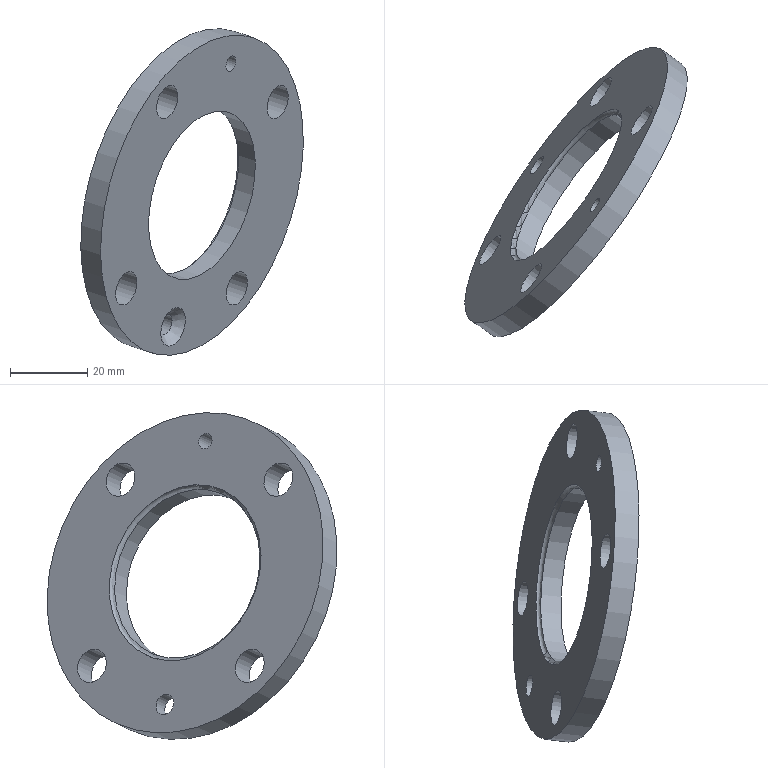Part | NX | features 2 2 | 1 solid | 12 faces | box 57.733 x 75.196 x 84.752 mm | volume 25201 mm3 | cylinder 8 | plane 2 | torus 1 | cone 1 | commonest cylinder face diameters 9 x4 4.2 x1 5.5 x1 45.3 x1 86 x1
STEP:
#1=CARTESIAN_POINT('',(-585.248,627.093,69.543));
#2=VERTEX_POINT('',#1);
#3=CARTESIAN_POINT('',(-609.911,591.869,69.543));
#4=DIRECTION('',(-0.7912,0.554,0.2588));
#5=DIRECTION('',(0.5736,0.8192,0.));
#6=AXIS2_PLACEMENT_3D('',#3,#4,#5);
#7=CIRCLE('',#6,43.);
#8=EDGE_CURVE('',#2,#2,#7,.T.);
#9=ORIENTED_EDGE('',*,*,#8,.F.);
#10=EDGE_LOOP('',(#9));
#11=FACE_BOUND('',#10,.T.);
#12=CARTESIAN_POINT('',(-580.105,623.491,67.86));
#13=VERTEX_POINT('',#12);
#14=CARTESIAN_POINT('',(-604.768,588.268,67.86));
#15=DIRECTION('',(0.7912,-0.554,-0.2588));
#16=DIRECTION('',(0.5736,0.8192,0.));
#17=AXIS2_PLACEMENT_3D('',#14,#15,#16);
#18=CIRCLE('',#17,43.);
#19=EDGE_CURVE('',#13,#13,#18,.T.);
#20=ORIENTED_EDGE('',*,*,#19,.F.);
#21=EDGE_LOOP('',(#20));
#22=FACE_BOUND('',#21,.T.);
#23=CARTESIAN_POINT('',(-609.911,591.869,69.543));
#24=DIRECTION('',(-0.7912,0.554,0.2588));
#25=DIRECTION('',(-0.5736,-0.8192,0.));
#26=AXIS2_PLACEMENT_3D('',#23,#24,#25);
#27=CYLINDRICAL_SURFACE('',#26,43.);
#28=ADVANCED_FACE('',(#11,#22),#27,.T.);
#29=CARTESIAN_POINT('',(-596.129,609.869,69.284));
#30=VERTEX_POINT('',#29);
#31=CARTESIAN_POINT('',(-609.12,591.315,69.284));
#32=DIRECTION('',(0.7912,-0.554,-0.2588));
#33=DIRECTION('',(0.5736,0.8192,0.));
#34=AXIS2_PLACEMENT_3D('',#31,#32,#33);
#35=CIRCLE('',#34,22.65);
#36=EDGE_CURVE('',#30,#30,#35,.T.);
#37=ORIENTED_EDGE('',*,*,#36,.F.);
#38=EDGE_LOOP('',(#37));
#39=FACE_BOUND('',#38,.T.);
#40=CARTESIAN_POINT('',(-591.777,606.822,67.86));
#41=VERTEX_POINT('',#40);
#42=CARTESIAN_POINT('',(-604.768,588.268,67.86));
#43=DIRECTION('',(0.7912,-0.554,-0.2588));
#44=DIRECTION('',(0.5736,0.8192,0.));
#45=AXIS2_PLACEMENT_3D('',#42,#43,#44);
#46=CIRCLE('',#45,22.65);
#47=EDGE_CURVE('',#41,#41,#46,.T.);
#48=ORIENTED_EDGE('',*,*,#47,.T.);
#49=EDGE_LOOP('',(#48));
#50=FACE_BOUND('',#49,.T.);
#51=CARTESIAN_POINT('',(-594.482,581.066,64.496));
#52=DIRECTION('',(0.7912,-0.554,-0.2588));
#53=DIRECTION('',(0.5736,0.8192,0.));
#54=AXIS2_PLACEMENT_3D('',#51,#52,#53);
#55=CYLINDRICAL_SURFACE('',#54,22.65);
#56=ADVANCED_FACE('',(#39,#50),#55,.F.);
#57=CARTESIAN_POINT('',(-626.97,578.788,45.395));
#58=VERTEX_POINT('',#57);
#59=CARTESIAN_POINT('',(-629.551,575.102,45.395));
#60=DIRECTION('',(-0.7912,0.554,0.2588));
#61=DIRECTION('',(0.5736,0.8192,0.));
#62=AXIS2_PLACEMENT_3D('',#59,#60,#61);
#63=CIRCLE('',#62,4.5);
#64=EDGE_CURVE('',#58,#58,#63,.T.);
#65=ORIENTED_EDGE('',*,*,#64,.T.);
#66=EDGE_LOOP('',(#65));
#67=FACE_BOUND('',#66,.T.);
#68=CARTESIAN_POINT('',(-621.827,575.187,43.712));
#69=VERTEX_POINT('',#68);
#70=CARTESIAN_POINT('',(-624.408,571.5,43.712));
#71=DIRECTION('',(0.7912,-0.554,-0.2588));
#72=DIRECTION('',(0.5736,0.8192,0.));
#73=AXIS2_PLACEMENT_3D('',#70,#71,#72);
#74=CIRCLE('',#73,4.5);
#75=EDGE_CURVE('',#69,#69,#74,.T.);
#76=ORIENTED_EDGE('',*,*,#75,.T.);
#77=EDGE_LOOP('',(#76));
#78=FACE_BOUND('',#77,.T.);
#79=CARTESIAN_POINT('',(-614.122,564.298,40.348));
#80=DIRECTION('',(0.7912,-0.554,-0.2588));
#81=DIRECTION('',(0.5736,0.8192,0.));
#82=AXIS2_PLACEMENT_3D('',#79,#80,#81);
#83=CYLINDRICAL_SURFACE('',#82,4.5);
#84=ADVANCED_FACE('',(#67,#78),#83,.F.);
#85=CARTESIAN_POINT('',(-616.369,571.365,93.691));
#86=VERTEX_POINT('',#85);
#87=CARTESIAN_POINT('',(-618.951,567.679,93.691));
#88=DIRECTION('',(-0.7912,0.554,0.2588));
#89=DIRECTION('',(0.5736,0.8192,0.));
#90=AXIS2_PLACEMENT_3D('',#87,#88,#89);
#91=CIRCLE('',#90,4.5);
#92=EDGE_CURVE('',#86,#86,#91,.T.);
#93=ORIENTED_EDGE('',*,*,#92,.T.);
#94=EDGE_LOOP('',(#93));
#95=FACE_BOUND('',#94,.T.);
#96=CARTESIAN_POINT('',(-611.226,567.764,92.009));
#97=VERTEX_POINT('',#96);
#98=CARTESIAN_POINT('',(-613.807,564.078,92.009));
#99=DIRECTION('',(0.7912,-0.554,-0.2588));
#100=DIRECTION('',(0.5736,0.8192,0.));
#101=AXIS2_PLACEMENT_3D('',#98,#99,#100);
#102=CIRCLE('',#101,4.5);
#103=EDGE_CURVE('',#97,#97,#102,.T.);
#104=ORIENTED_EDGE('',*,*,#103,.T.);
#105=EDGE_LOOP('',(#104));
#106=FACE_BOUND('',#105,.T.);
#107=CARTESIAN_POINT('',(-603.521,556.875,88.644));
#108=DIRECTION('',(0.7912,-0.554,-0.2588));
#109=DIRECTION('',(0.5736,0.8192,0.));
#110=AXIS2_PLACEMENT_3D('',#107,#108,#109);
#111=CYLINDRICAL_SURFACE('',#110,4.5);
#112=ADVANCED_FACE('',(#95,#106),#111,.F.);
#113=CARTESIAN_POINT('',(-598.291,619.745,45.395));
#114=VERTEX_POINT('',#113);
#115=CARTESIAN_POINT('',(-600.872,616.059,45.395));
#116=DIRECTION('',(-0.7912,0.554,0.2588));
#117=DIRECTION('',(0.5736,0.8192,0.));
#118=AXIS2_PLACEMENT_3D('',#115,#116,#117);
#119=CIRCLE('',#118,4.5);
#120=EDGE_CURVE('',#114,#114,#119,.T.);
#121=ORIENTED_EDGE('',*,*,#120,.T.);
#122=EDGE_LOOP('',(#121));
#123=FACE_BOUND('',#122,.T.);
#124=CARTESIAN_POINT('',(-593.148,616.144,43.712));
#125=VERTEX_POINT('',#124);
#126=CARTESIAN_POINT('',(-595.729,612.458,43.712));
#127=DIRECTION('',(0.7912,-0.554,-0.2588));
#128=DIRECTION('',(0.5736,0.8192,0.));
#129=AXIS2_PLACEMENT_3D('',#126,#127,#128);
#130=CIRCLE('',#129,4.5);
#131=EDGE_CURVE('',#125,#125,#130,.T.);
#132=ORIENTED_EDGE('',*,*,#131,.T.);
#133=EDGE_LOOP('',(#132));
#134=FACE_BOUND('',#133,.T.);
#135=CARTESIAN_POINT('',(-585.443,605.256,40.348));
#136=DIRECTION('',(0.7912,-0.554,-0.2588));
#137=DIRECTION('',(0.5736,0.8192,0.));
#138=AXIS2_PLACEMENT_3D('',#135,#136,#137);
#139=CYLINDRICAL_SURFACE('',#138,4.5);
#140=ADVANCED_FACE('',(#123,#134),#139,.F.);
#141=CARTESIAN_POINT('',(-587.691,612.323,93.691));
#142=VERTEX_POINT('',#141);
#143=CARTESIAN_POINT('',(-590.272,608.637,93.691));
#144=DIRECTION('',(-0.7912,0.554,0.2588));
#145=DIRECTION('',(0.5736,0.8192,0.));
#146=AXIS2_PLACEMENT_3D('',#143,#144,#145);
#147=CIRCLE('',#146,4.5);
#148=EDGE_CURVE('',#142,#142,#147,.T.);
#149=ORIENTED_EDGE('',*,*,#148,.T.);
#150=EDGE_LOOP('',(#149));
#151=FACE_BOUND('',#150,.T.);
#152=CARTESIAN_POINT('',(-582.548,608.722,92.009));
#153=VERTEX_POINT('',#152);
#154=CARTESIAN_POINT('',(-585.129,605.035,92.009));
#155=DIRECTION('',(0.7912,-0.554,-0.2588));
#156=DIRECTION('',(0.5736,0.8192,0.));
#157=AXIS2_PLACEMENT_3D('',#154,#155,#156);
#158=CIRCLE('',#157,4.5);
#159=EDGE_CURVE('',#153,#153,#158,.T.);
#160=ORIENTED_EDGE('',*,*,#159,.T.);
#161=EDGE_LOOP('',(#160));
#162=FACE_BOUND('',#161,.T.);
#163=CARTESIAN_POINT('',(-574.843,597.833,88.644));
#164=DIRECTION('',(0.7912,-0.554,-0.2588));
#165=DIRECTION('',(0.5736,0.8192,0.));
#166=AXIS2_PLACEMENT_3D('',#163,#164,#165);
#167=CYLINDRICAL_SURFACE('',#166,4.5);
#168=ADVANCED_FACE('',(#151,#162),#167,.F.);
#169=CARTESIAN_POINT('',(-623.477,572.496,69.543));
#170=VERTEX_POINT('',#169);
#171=CARTESIAN_POINT('',(-609.911,591.869,69.543));
#172=DIRECTION('',(-0.7912,0.554,0.2588));
#173=DIRECTION('',(-0.5736,-0.8192,0.));
#174=AXIS2_PLACEMENT_3D('',#171,#172,#173);
#175=CIRCLE('',#174,23.65);
#176=EDGE_CURVE('',#170,#170,#175,.T.);
#177=ORIENTED_EDGE('',*,*,#176,.T.);
#178=EDGE_LOOP('',(#177));
#179=FACE_BOUND('',#178,.T.);
#180=ORIENTED_EDGE('',*,*,#36,.T.);
#181=EDGE_LOOP('',(#180));
#182=FACE_BOUND('',#181,.T.);
#183=CARTESIAN_POINT('',(-609.911,591.869,69.543));
#184=DIRECTION('',(-0.7912,0.554,0.2588));
#185=DIRECTION('',(-0.5736,-0.8192,0.));
#186=AXIS2_PLACEMENT_3D('',#183,#184,#185);
#187=TOROIDAL_SURFACE('',#186,22.65,1.);
#188=ADVANCED_FACE('',(#179,#182),#187,.F.);
#189=CARTESIAN_POINT('',(-613.365,594.288,28.692));
#190=VERTEX_POINT('',#189);
#191=CARTESIAN_POINT('',(-612.263,593.516,33.715));
#192=DIRECTION('',(0.7912,-0.554,-0.2588));
#193=DIRECTION('',(-0.212,0.1485,-0.9659));
#194=AXIS2_PLACEMENT_3D('',#191,#192,#193);
#195=CIRCLE('',#194,5.2);
#196=EDGE_CURVE('',#190,#190,#195,.T.);
#197=ORIENTED_EDGE('',*,*,#196,.T.);
#198=EDGE_LOOP('',(#197));
#199=FACE_BOUND('',#198,.T.);
#200=CARTESIAN_POINT('',(-614.785,595.281,31.693));
#201=VERTEX_POINT('',#200);
#202=CARTESIAN_POINT('',(-614.202,594.873,34.349));
#203=DIRECTION('',(-0.7912,0.554,0.2588));
#204=DIRECTION('',(-0.212,0.1485,-0.9659));
#205=AXIS2_PLACEMENT_3D('',#202,#203,#204);
#206=CIRCLE('',#205,2.75);
#207=EDGE_CURVE('',#201,#201,#206,.T.);
#208=ORIENTED_EDGE('',*,*,#207,.T.);
#209=EDGE_LOOP('',(#208));
#210=FACE_BOUND('',#209,.T.);
#211=CARTESIAN_POINT('',(-613.232,594.194,34.032));
#212=DIRECTION('',(0.7912,-0.554,-0.2588));
#213=DIRECTION('',(0.5736,0.8192,0.));
#214=AXIS2_PLACEMENT_3D('',#211,#212,#213);
#215=CONICAL_SURFACE('',#214,3.975,0.7854);
#216=ADVANCED_FACE('',(#199,#210),#215,.F.);
#217=ORIENTED_EDGE('',*,*,#207,.F.);
#218=EDGE_LOOP('',(#217));
#219=FACE_BOUND('',#218,.T.);
#220=CARTESIAN_POINT('',(-617.989,597.525,32.741));
#221=VERTEX_POINT('',#220);
#222=CARTESIAN_POINT('',(-617.406,597.117,35.397));
#223=DIRECTION('',(-0.7912,0.554,0.2588));
#224=DIRECTION('',(-0.212,0.1485,-0.9659));
#225=AXIS2_PLACEMENT_3D('',#222,#223,#224);
#226=CIRCLE('',#225,2.75);
#227=EDGE_CURVE('',#221,#221,#226,.T.);
#228=ORIENTED_EDGE('',*,*,#227,.T.);
#229=EDGE_LOOP('',(#228));
#230=FACE_BOUND('',#229,.T.);
#231=CARTESIAN_POINT('',(-615.804,595.995,34.873));
#232=DIRECTION('',(-0.7912,0.554,0.2588));
#233=DIRECTION('',(-0.5736,-0.8192,0.));
#234=AXIS2_PLACEMENT_3D('',#231,#232,#233);
#235=CYLINDRICAL_SURFACE('',#234,2.75);
#236=ADVANCED_FACE('',(#219,#230),#235,.F.);
#237=CARTESIAN_POINT('',(-601.972,586.31,105.717));
#238=VERTEX_POINT('',#237);
#239=CARTESIAN_POINT('',(-602.417,586.621,103.688));
#240=DIRECTION('',(-0.7912,0.554,0.2588));
#241=DIRECTION('',(0.212,-0.1485,0.9659));
#242=AXIS2_PLACEMENT_3D('',#239,#240,#241);
#243=CIRCLE('',#242,2.1);
#244=EDGE_CURVE('',#238,#238,#243,.T.);
#245=ORIENTED_EDGE('',*,*,#244,.T.);
#246=EDGE_LOOP('',(#245));
#247=FACE_BOUND('',#246,.T.);
#248=CARTESIAN_POINT('',(-596.829,582.708,104.034));
#249=VERTEX_POINT('',#248);
#250=CARTESIAN_POINT('',(-597.274,583.02,102.006));
#251=DIRECTION('',(0.7912,-0.554,-0.2588));
#252=DIRECTION('',(0.212,-0.1485,0.9659));
#253=AXIS2_PLACEMENT_3D('',#250,#251,#252);
#254=CIRCLE('',#253,2.1);
#255=EDGE_CURVE('',#249,#249,#254,.T.);
#256=ORIENTED_EDGE('',*,*,#255,.T.);
#257=EDGE_LOOP('',(#256));
#258=FACE_BOUND('',#257,.T.);
#259=CARTESIAN_POINT('',(-599.845,584.821,102.847));
#260=DIRECTION('',(0.7912,-0.554,-0.2588));
#261=DIRECTION('',(0.5736,0.8192,0.));
#262=AXIS2_PLACEMENT_3D('',#259,#260,#261);
#263=CYLINDRICAL_SURFACE('',#262,2.1);
#264=ADVANCED_FACE('',(#247,#258),#263,.F.);
#265=ORIENTED_EDGE('',*,*,#255,.F.);
#266=EDGE_LOOP('',(#265));
#267=FACE_BOUND('',#266,.T.);
#268=ORIENTED_EDGE('',*,*,#196,.F.);
#269=EDGE_LOOP('',(#268));
#270=FACE_BOUND('',#269,.T.);
#271=ORIENTED_EDGE('',*,*,#159,.F.);
#272=EDGE_LOOP('',(#271));
#273=FACE_BOUND('',#272,.T.);
#274=ORIENTED_EDGE('',*,*,#131,.F.);
#275=EDGE_LOOP('',(#274));
#276=FACE_BOUND('',#275,.T.);
#277=ORIENTED_EDGE('',*,*,#103,.F.);
#278=EDGE_LOOP('',(#277));
#279=FACE_BOUND('',#278,.T.);
#280=ORIENTED_EDGE('',*,*,#75,.F.);
#281=EDGE_LOOP('',(#280));
#282=FACE_BOUND('',#281,.T.);
#283=ORIENTED_EDGE('',*,*,#47,.F.);
#284=EDGE_LOOP('',(#283));
#285=FACE_BOUND('',#284,.T.);
#286=ORIENTED_EDGE('',*,*,#19,.T.);
#287=EDGE_LOOP('',(#286));
#288=FACE_BOUND('',#287,.T.);
#289=CARTESIAN_POINT('',(-604.768,588.268,67.86));
#290=DIRECTION('',(0.7912,-0.554,-0.2588));
#291=DIRECTION('',(0.5736,0.8192,0.));
#292=AXIS2_PLACEMENT_3D('',#289,#290,#291);
#293=PLANE('',#292);
#294=ADVANCED_FACE('',(#267,#270,#273,#276,#279,#282,#285,#288),#293,.T.);
#295=ORIENTED_EDGE('',*,*,#244,.F.);
#296=EDGE_LOOP('',(#295));
#297=FACE_BOUND('',#296,.T.);
#298=ORIENTED_EDGE('',*,*,#227,.F.);
#299=EDGE_LOOP('',(#298));
#300=FACE_BOUND('',#299,.T.);
#301=ORIENTED_EDGE('',*,*,#176,.F.);
#302=EDGE_LOOP('',(#301));
#303=FACE_BOUND('',#302,.T.);
#304=ORIENTED_EDGE('',*,*,#148,.F.);
#305=EDGE_LOOP('',(#304));
#306=FACE_BOUND('',#305,.T.);
#307=ORIENTED_EDGE('',*,*,#120,.F.);
#308=EDGE_LOOP('',(#307));
#309=FACE_BOUND('',#308,.T.);
#310=ORIENTED_EDGE('',*,*,#92,.F.);
#311=EDGE_LOOP('',(#310));
#312=FACE_BOUND('',#311,.T.);
#313=ORIENTED_EDGE('',*,*,#64,.F.);
#314=EDGE_LOOP('',(#313));
#315=FACE_BOUND('',#314,.T.);
#316=ORIENTED_EDGE('',*,*,#8,.T.);
#317=EDGE_LOOP('',(#316));
#318=FACE_BOUND('',#317,.T.);
#319=CARTESIAN_POINT('',(-609.911,591.869,69.543));
#320=DIRECTION('',(0.7912,-0.554,-0.2588));
#321=DIRECTION('',(0.5736,0.8192,0.));
#322=AXIS2_PLACEMENT_3D('',#319,#320,#321);
#323=PLANE('',#322);
#324=ADVANCED_FACE('',(#297,#300,#303,#306,#309,#312,#315,#318),#323,.F.);
#325=CLOSED_SHELL('',(#28,#56,#84,#112,#140,#168,#188,#216,#236,#264,#294,#324));
#326=MANIFOLD_SOLID_BREP('',#325);
#327=(LENGTH_UNIT()NAMED_UNIT(*)SI_UNIT(.MILLI.,.METRE.));
#328=UNCERTAINTY_MEASURE_WITH_UNIT(LENGTH_MEASURE(0.00001),#327,'','');
#329=(NAMED_UNIT(*)PLANE_ANGLE_UNIT()SI_UNIT($,.RADIAN.));
#330=(NAMED_UNIT(*)SI_UNIT($,.STERADIAN.)SOLID_ANGLE_UNIT());
#331=(GEOMETRIC_REPRESENTATION_CONTEXT(3)GLOBAL_UNCERTAINTY_ASSIGNED_CONTEXT((#328))GLOBAL_UNIT_ASSIGNED_CONTEXT((#327,#329,#330))REPRESENTATION_CONTEXT('',''));
#332=ADVANCED_BREP_SHAPE_REPRESENTATION('',(#326),#331);